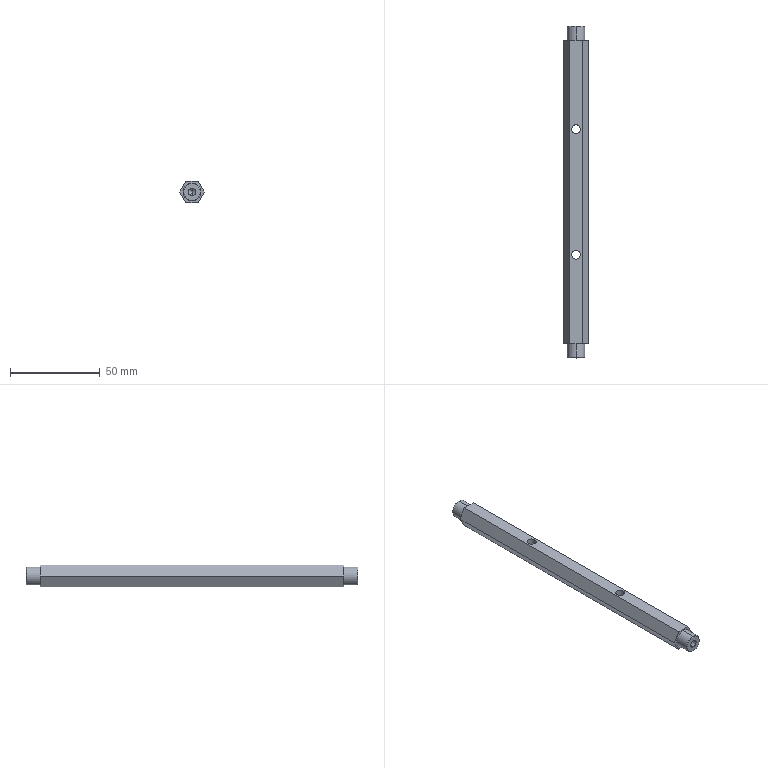Part | STEP file | PN_0002_default | 1 solid | 30 faces | box 13.856 x 185 x 12 mm | volume 21503 mm3 | cylinder 12 | plane 10 | cone 8 | commonest cylinder face diameters 4.2 x4 5 x4 10 x4